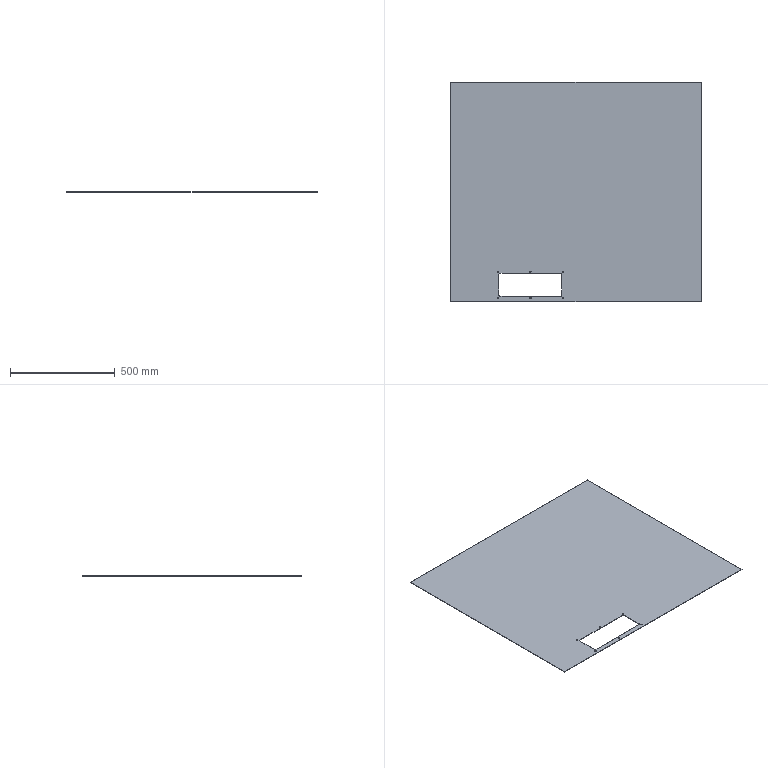Part | SolidWorks | features BaseBody 1 | 1 solid | 26 faces | box 1196 x 1046 x 2 mm | volume 2435677 mm3 | cylinder 16 | plane 10 | commonest cylinder face diameters 6.5 x12 10 x4
STEP:
#1=CARTESIAN_POINT('',(-369.75,-505.5,2.));
#2=VERTEX_POINT('',#1);
#3=CARTESIAN_POINT('',(-369.75,-505.5,0.));
#4=VERTEX_POINT('',#3);
#5=CARTESIAN_POINT('',(-369.75,-505.5,2.));
#6=DIRECTION('',(0.,0.,-1.));
#7=VECTOR('',#6,1000.);
#8=LINE('',#5,#7);
#9=EDGE_CURVE('',#2,#4,#8,.T.);
#10=ORIENTED_EDGE('',*,*,#9,.F.);
#11=CARTESIAN_POINT('',(-376.25,-505.5,2.));
#12=VERTEX_POINT('',#11);
#13=CARTESIAN_POINT('',(-373.,-505.5,2.));
#14=DIRECTION('',(0.,0.,-1.));
#15=DIRECTION('',(1.,0.,0.));
#16=AXIS2_PLACEMENT_3D('',#13,#14,#15);
#17=CIRCLE('',#16,3.25);
#18=EDGE_CURVE('',#12,#2,#17,.T.);
#19=ORIENTED_EDGE('',*,*,#18,.F.);
#20=CARTESIAN_POINT('',(-376.25,-505.5,0.));
#21=VERTEX_POINT('',#20);
#22=CARTESIAN_POINT('',(-376.25,-505.5,2.));
#23=DIRECTION('',(0.,0.,-1.));
#24=VECTOR('',#23,1000.);
#25=LINE('',#22,#24);
#26=EDGE_CURVE('',#12,#21,#25,.T.);
#27=ORIENTED_EDGE('',*,*,#26,.T.);
#28=CARTESIAN_POINT('',(-373.,-505.5,0.));
#29=DIRECTION('',(0.,0.,-1.));
#30=DIRECTION('',(1.,0.,0.));
#31=AXIS2_PLACEMENT_3D('',#28,#29,#30);
#32=CIRCLE('',#31,3.25);
#33=EDGE_CURVE('',#21,#4,#32,.T.);
#34=ORIENTED_EDGE('',*,*,#33,.T.);
#35=EDGE_LOOP('',(#10,#19,#27,#34));
#36=FACE_OUTER_BOUND('',#35,.T.);
#37=CARTESIAN_POINT('',(-373.,-505.5,2.));
#38=DIRECTION('',(0.,0.,-1.));
#39=DIRECTION('',(-1.,0.,0.));
#40=AXIS2_PLACEMENT_3D('',#37,#38,#39);
#41=CYLINDRICAL_SURFACE('',#40,3.25);
#42=ADVANCED_FACE('',(#36),#41,.F.);
#43=CARTESIAN_POINT('',(-214.75,-505.5,2.));
#44=VERTEX_POINT('',#43);
#45=CARTESIAN_POINT('',(-214.75,-505.5,0.));
#46=VERTEX_POINT('',#45);
#47=CARTESIAN_POINT('',(-214.75,-505.5,2.));
#48=DIRECTION('',(0.,0.,-1.));
#49=VECTOR('',#48,1000.);
#50=LINE('',#47,#49);
#51=EDGE_CURVE('',#44,#46,#50,.T.);
#52=ORIENTED_EDGE('',*,*,#51,.F.);
#53=CARTESIAN_POINT('',(-221.25,-505.5,2.));
#54=VERTEX_POINT('',#53);
#55=CARTESIAN_POINT('',(-218.,-505.5,2.));
#56=DIRECTION('',(0.,0.,-1.));
#57=DIRECTION('',(-1.,0.,0.));
#58=AXIS2_PLACEMENT_3D('',#55,#56,#57);
#59=CIRCLE('',#58,3.25);
#60=EDGE_CURVE('',#54,#44,#59,.T.);
#61=ORIENTED_EDGE('',*,*,#60,.F.);
#62=CARTESIAN_POINT('',(-221.25,-505.5,0.));
#63=VERTEX_POINT('',#62);
#64=CARTESIAN_POINT('',(-221.25,-505.5,2.));
#65=DIRECTION('',(0.,0.,-1.));
#66=VECTOR('',#65,1000.);
#67=LINE('',#64,#66);
#68=EDGE_CURVE('',#54,#63,#67,.T.);
#69=ORIENTED_EDGE('',*,*,#68,.T.);
#70=CARTESIAN_POINT('',(-218.,-505.5,0.));
#71=DIRECTION('',(0.,0.,-1.));
#72=DIRECTION('',(-1.,0.,0.));
#73=AXIS2_PLACEMENT_3D('',#70,#71,#72);
#74=CIRCLE('',#73,3.25);
#75=EDGE_CURVE('',#63,#46,#74,.T.);
#76=ORIENTED_EDGE('',*,*,#75,.T.);
#77=EDGE_LOOP('',(#52,#61,#69,#76));
#78=FACE_OUTER_BOUND('',#77,.T.);
#79=CARTESIAN_POINT('',(-218.,-505.5,2.));
#80=DIRECTION('',(0.,0.,-1.));
#81=DIRECTION('',(-1.,0.,0.));
#82=AXIS2_PLACEMENT_3D('',#79,#80,#81);
#83=CYLINDRICAL_SURFACE('',#82,3.25);
#84=ADVANCED_FACE('',(#78),#83,.F.);
#85=CARTESIAN_POINT('',(-214.75,-380.5,2.));
#86=VERTEX_POINT('',#85);
#87=CARTESIAN_POINT('',(-214.75,-380.5,0.));
#88=VERTEX_POINT('',#87);
#89=CARTESIAN_POINT('',(-214.75,-380.5,2.));
#90=DIRECTION('',(0.,0.,-1.));
#91=VECTOR('',#90,1000.);
#92=LINE('',#89,#91);
#93=EDGE_CURVE('',#86,#88,#92,.T.);
#94=ORIENTED_EDGE('',*,*,#93,.F.);
#95=CARTESIAN_POINT('',(-221.25,-380.5,2.));
#96=VERTEX_POINT('',#95);
#97=CARTESIAN_POINT('',(-218.,-380.5,2.));
#98=DIRECTION('',(0.,0.,-1.));
#99=DIRECTION('',(-1.,0.,0.));
#100=AXIS2_PLACEMENT_3D('',#97,#98,#99);
#101=CIRCLE('',#100,3.25);
#102=EDGE_CURVE('',#96,#86,#101,.T.);
#103=ORIENTED_EDGE('',*,*,#102,.F.);
#104=CARTESIAN_POINT('',(-221.25,-380.5,0.));
#105=VERTEX_POINT('',#104);
#106=CARTESIAN_POINT('',(-221.25,-380.5,2.));
#107=DIRECTION('',(0.,0.,-1.));
#108=VECTOR('',#107,1000.);
#109=LINE('',#106,#108);
#110=EDGE_CURVE('',#96,#105,#109,.T.);
#111=ORIENTED_EDGE('',*,*,#110,.T.);
#112=CARTESIAN_POINT('',(-218.,-380.5,0.));
#113=DIRECTION('',(0.,0.,-1.));
#114=DIRECTION('',(-1.,0.,0.));
#115=AXIS2_PLACEMENT_3D('',#112,#113,#114);
#116=CIRCLE('',#115,3.25);
#117=EDGE_CURVE('',#105,#88,#116,.T.);
#118=ORIENTED_EDGE('',*,*,#117,.T.);
#119=EDGE_LOOP('',(#94,#103,#111,#118));
#120=FACE_OUTER_BOUND('',#119,.T.);
#121=CARTESIAN_POINT('',(-218.,-380.5,2.));
#122=DIRECTION('',(0.,0.,-1.));
#123=DIRECTION('',(-1.,0.,0.));
#124=AXIS2_PLACEMENT_3D('',#121,#122,#123);
#125=CYLINDRICAL_SURFACE('',#124,3.25);
#126=ADVANCED_FACE('',(#120),#125,.F.);
#127=CARTESIAN_POINT('',(-59.75,-505.5,2.));
#128=VERTEX_POINT('',#127);
#129=CARTESIAN_POINT('',(-59.75,-505.5,0.));
#130=VERTEX_POINT('',#129);
#131=CARTESIAN_POINT('',(-59.75,-505.5,2.));
#132=DIRECTION('',(0.,0.,-1.));
#133=VECTOR('',#132,1000.);
#134=LINE('',#131,#133);
#135=EDGE_CURVE('',#128,#130,#134,.T.);
#136=ORIENTED_EDGE('',*,*,#135,.F.);
#137=CARTESIAN_POINT('',(-66.25,-505.5,2.));
#138=VERTEX_POINT('',#137);
#139=CARTESIAN_POINT('',(-63.,-505.5,2.));
#140=DIRECTION('',(0.,0.,-1.));
#141=DIRECTION('',(-1.,0.,0.));
#142=AXIS2_PLACEMENT_3D('',#139,#140,#141);
#143=CIRCLE('',#142,3.25);
#144=EDGE_CURVE('',#138,#128,#143,.T.);
#145=ORIENTED_EDGE('',*,*,#144,.F.);
#146=CARTESIAN_POINT('',(-66.25,-505.5,0.));
#147=VERTEX_POINT('',#146);
#148=CARTESIAN_POINT('',(-66.25,-505.5,2.));
#149=DIRECTION('',(0.,0.,-1.));
#150=VECTOR('',#149,1000.);
#151=LINE('',#148,#150);
#152=EDGE_CURVE('',#138,#147,#151,.T.);
#153=ORIENTED_EDGE('',*,*,#152,.T.);
#154=CARTESIAN_POINT('',(-63.,-505.5,0.));
#155=DIRECTION('',(0.,0.,-1.));
#156=DIRECTION('',(-1.,0.,0.));
#157=AXIS2_PLACEMENT_3D('',#154,#155,#156);
#158=CIRCLE('',#157,3.25);
#159=EDGE_CURVE('',#147,#130,#158,.T.);
#160=ORIENTED_EDGE('',*,*,#159,.T.);
#161=EDGE_LOOP('',(#136,#145,#153,#160));
#162=FACE_OUTER_BOUND('',#161,.T.);
#163=CARTESIAN_POINT('',(-63.,-505.5,2.));
#164=DIRECTION('',(0.,0.,-1.));
#165=DIRECTION('',(-1.,0.,0.));
#166=AXIS2_PLACEMENT_3D('',#163,#164,#165);
#167=CYLINDRICAL_SURFACE('',#166,3.25);
#168=ADVANCED_FACE('',(#162),#167,.F.);
#169=CARTESIAN_POINT('',(-369.75,-380.5,2.));
#170=VERTEX_POINT('',#169);
#171=CARTESIAN_POINT('',(-369.75,-380.5,0.));
#172=VERTEX_POINT('',#171);
#173=CARTESIAN_POINT('',(-369.75,-380.5,2.));
#174=DIRECTION('',(0.,0.,-1.));
#175=VECTOR('',#174,1000.);
#176=LINE('',#173,#175);
#177=EDGE_CURVE('',#170,#172,#176,.T.);
#178=ORIENTED_EDGE('',*,*,#177,.F.);
#179=CARTESIAN_POINT('',(-376.25,-380.5,2.));
#180=VERTEX_POINT('',#179);
#181=CARTESIAN_POINT('',(-373.,-380.5,2.));
#182=DIRECTION('',(0.,0.,-1.));
#183=DIRECTION('',(1.,0.,0.));
#184=AXIS2_PLACEMENT_3D('',#181,#182,#183);
#185=CIRCLE('',#184,3.25);
#186=EDGE_CURVE('',#180,#170,#185,.T.);
#187=ORIENTED_EDGE('',*,*,#186,.F.);
#188=CARTESIAN_POINT('',(-376.25,-380.5,0.));
#189=VERTEX_POINT('',#188);
#190=CARTESIAN_POINT('',(-376.25,-380.5,2.));
#191=DIRECTION('',(0.,0.,-1.));
#192=VECTOR('',#191,1000.);
#193=LINE('',#190,#192);
#194=EDGE_CURVE('',#180,#189,#193,.T.);
#195=ORIENTED_EDGE('',*,*,#194,.T.);
#196=CARTESIAN_POINT('',(-373.,-380.5,0.));
#197=DIRECTION('',(0.,0.,-1.));
#198=DIRECTION('',(1.,0.,0.));
#199=AXIS2_PLACEMENT_3D('',#196,#197,#198);
#200=CIRCLE('',#199,3.25);
#201=EDGE_CURVE('',#189,#172,#200,.T.);
#202=ORIENTED_EDGE('',*,*,#201,.T.);
#203=EDGE_LOOP('',(#178,#187,#195,#202));
#204=FACE_OUTER_BOUND('',#203,.T.);
#205=CARTESIAN_POINT('',(-373.,-380.5,2.));
#206=DIRECTION('',(0.,0.,-1.));
#207=DIRECTION('',(-1.,0.,0.));
#208=AXIS2_PLACEMENT_3D('',#205,#206,#207);
#209=CYLINDRICAL_SURFACE('',#208,3.25);
#210=ADVANCED_FACE('',(#204),#209,.F.);
#211=CARTESIAN_POINT('',(-59.75,-380.5,2.));
#212=VERTEX_POINT('',#211);
#213=CARTESIAN_POINT('',(-59.75,-380.5,0.));
#214=VERTEX_POINT('',#213);
#215=CARTESIAN_POINT('',(-59.75,-380.5,2.));
#216=DIRECTION('',(0.,0.,-1.));
#217=VECTOR('',#216,1000.);
#218=LINE('',#215,#217);
#219=EDGE_CURVE('',#212,#214,#218,.T.);
#220=ORIENTED_EDGE('',*,*,#219,.F.);
#221=CARTESIAN_POINT('',(-66.25,-380.5,2.));
#222=VERTEX_POINT('',#221);
#223=CARTESIAN_POINT('',(-63.,-380.5,2.));
#224=DIRECTION('',(0.,0.,-1.));
#225=DIRECTION('',(-1.,0.,0.));
#226=AXIS2_PLACEMENT_3D('',#223,#224,#225);
#227=CIRCLE('',#226,3.25);
#228=EDGE_CURVE('',#222,#212,#227,.T.);
#229=ORIENTED_EDGE('',*,*,#228,.F.);
#230=CARTESIAN_POINT('',(-66.25,-380.5,0.));
#231=VERTEX_POINT('',#230);
#232=CARTESIAN_POINT('',(-66.25,-380.5,2.));
#233=DIRECTION('',(0.,0.,-1.));
#234=VECTOR('',#233,1000.);
#235=LINE('',#232,#234);
#236=EDGE_CURVE('',#222,#231,#235,.T.);
#237=ORIENTED_EDGE('',*,*,#236,.T.);
#238=CARTESIAN_POINT('',(-63.,-380.5,0.));
#239=DIRECTION('',(0.,0.,-1.));
#240=DIRECTION('',(-1.,0.,0.));
#241=AXIS2_PLACEMENT_3D('',#238,#239,#240);
#242=CIRCLE('',#241,3.25);
#243=EDGE_CURVE('',#231,#214,#242,.T.);
#244=ORIENTED_EDGE('',*,*,#243,.T.);
#245=EDGE_LOOP('',(#220,#229,#237,#244));
#246=FACE_OUTER_BOUND('',#245,.T.);
#247=CARTESIAN_POINT('',(-63.,-380.5,2.));
#248=DIRECTION('',(0.,0.,-1.));
#249=DIRECTION('',(-1.,0.,0.));
#250=AXIS2_PLACEMENT_3D('',#247,#248,#249);
#251=CYLINDRICAL_SURFACE('',#250,3.25);
#252=ADVANCED_FACE('',(#246),#251,.F.);
#253=CARTESIAN_POINT('',(-73.,-388.,2.));
#254=VERTEX_POINT('',#253);
#255=CARTESIAN_POINT('',(-68.,-393.,2.));
#256=VERTEX_POINT('',#255);
#257=CARTESIAN_POINT('',(-73.,-393.,2.));
#258=DIRECTION('',(0.,0.,-1.));
#259=DIRECTION('',(-1.,0.,0.));
#260=AXIS2_PLACEMENT_3D('',#257,#258,#259);
#261=CIRCLE('',#260,5.);
#262=EDGE_CURVE('',#254,#256,#261,.T.);
#263=ORIENTED_EDGE('',*,*,#262,.F.);
#264=CARTESIAN_POINT('',(-73.,-388.,0.));
#265=VERTEX_POINT('',#264);
#266=CARTESIAN_POINT('',(-73.,-388.,2.));
#267=DIRECTION('',(0.,0.,1.));
#268=VECTOR('',#267,1000.);
#269=LINE('',#266,#268);
#270=EDGE_CURVE('',#265,#254,#269,.T.);
#271=ORIENTED_EDGE('',*,*,#270,.F.);
#272=CARTESIAN_POINT('',(-68.,-393.,0.));
#273=VERTEX_POINT('',#272);
#274=CARTESIAN_POINT('',(-73.,-393.,0.));
#275=DIRECTION('',(0.,0.,1.));
#276=DIRECTION('',(-1.,0.,0.));
#277=AXIS2_PLACEMENT_3D('',#274,#275,#276);
#278=CIRCLE('',#277,5.);
#279=EDGE_CURVE('',#273,#265,#278,.T.);
#280=ORIENTED_EDGE('',*,*,#279,.F.);
#281=CARTESIAN_POINT('',(-68.,-393.,0.));
#282=DIRECTION('',(0.,0.,-1.));
#283=VECTOR('',#282,1000.);
#284=LINE('',#281,#283);
#285=EDGE_CURVE('',#256,#273,#284,.T.);
#286=ORIENTED_EDGE('',*,*,#285,.F.);
#287=EDGE_LOOP('',(#263,#271,#280,#286));
#288=FACE_OUTER_BOUND('',#287,.T.);
#289=CARTESIAN_POINT('',(-73.,-393.,10.));
#290=DIRECTION('',(0.,0.,1.));
#291=DIRECTION('',(1.,0.,0.));
#292=AXIS2_PLACEMENT_3D('',#289,#290,#291);
#293=CYLINDRICAL_SURFACE('',#292,5.);
#294=ADVANCED_FACE('',(#288),#293,.F.);
#295=CARTESIAN_POINT('',(-68.,-493.,2.));
#296=VERTEX_POINT('',#295);
#297=CARTESIAN_POINT('',(-73.,-498.,2.));
#298=VERTEX_POINT('',#297);
#299=CARTESIAN_POINT('',(-73.,-493.,2.));
#300=DIRECTION('',(0.,0.,-1.));
#301=DIRECTION('',(-1.,0.,0.));
#302=AXIS2_PLACEMENT_3D('',#299,#300,#301);
#303=CIRCLE('',#302,5.);
#304=EDGE_CURVE('',#296,#298,#303,.T.);
#305=ORIENTED_EDGE('',*,*,#304,.F.);
#306=CARTESIAN_POINT('',(-68.,-493.,0.));
#307=VERTEX_POINT('',#306);
#308=CARTESIAN_POINT('',(-68.,-493.,2.));
#309=DIRECTION('',(0.,0.,1.));
#310=VECTOR('',#309,1000.);
#311=LINE('',#308,#310);
#312=EDGE_CURVE('',#307,#296,#311,.T.);
#313=ORIENTED_EDGE('',*,*,#312,.F.);
#314=CARTESIAN_POINT('',(-73.,-498.,0.));
#315=VERTEX_POINT('',#314);
#316=CARTESIAN_POINT('',(-73.,-493.,0.));
#317=DIRECTION('',(0.,0.,1.));
#318=DIRECTION('',(-1.,0.,0.));
#319=AXIS2_PLACEMENT_3D('',#316,#317,#318);
#320=CIRCLE('',#319,5.);
#321=EDGE_CURVE('',#315,#307,#320,.T.);
#322=ORIENTED_EDGE('',*,*,#321,.F.);
#323=CARTESIAN_POINT('',(-73.,-498.,0.));
#324=DIRECTION('',(0.,0.,-1.));
#325=VECTOR('',#324,1000.);
#326=LINE('',#323,#325);
#327=EDGE_CURVE('',#298,#315,#326,.T.);
#328=ORIENTED_EDGE('',*,*,#327,.F.);
#329=EDGE_LOOP('',(#305,#313,#322,#328));
#330=FACE_OUTER_BOUND('',#329,.T.);
#331=CARTESIAN_POINT('',(-73.,-493.,10.));
#332=DIRECTION('',(0.,0.,1.));
#333=DIRECTION('',(1.,0.,0.));
#334=AXIS2_PLACEMENT_3D('',#331,#332,#333);
#335=CYLINDRICAL_SURFACE('',#334,5.);
#336=ADVANCED_FACE('',(#330),#335,.F.);
#337=CARTESIAN_POINT('',(-368.,-393.,2.));
#338=VERTEX_POINT('',#337);
#339=CARTESIAN_POINT('',(-363.,-388.,2.));
#340=VERTEX_POINT('',#339);
#341=CARTESIAN_POINT('',(-363.,-393.,2.));
#342=DIRECTION('',(0.,0.,-1.));
#343=DIRECTION('',(-1.,0.,0.));
#344=AXIS2_PLACEMENT_3D('',#341,#342,#343);
#345=CIRCLE('',#344,5.);
#346=EDGE_CURVE('',#338,#340,#345,.T.);
#347=ORIENTED_EDGE('',*,*,#346,.F.);
#348=CARTESIAN_POINT('',(-368.,-393.,0.));
#349=VERTEX_POINT('',#348);
#350=CARTESIAN_POINT('',(-368.,-393.,2.));
#351=DIRECTION('',(0.,0.,1.));
#352=VECTOR('',#351,1000.);
#353=LINE('',#350,#352);
#354=EDGE_CURVE('',#349,#338,#353,.T.);
#355=ORIENTED_EDGE('',*,*,#354,.F.);
#356=CARTESIAN_POINT('',(-363.,-388.,0.));
#357=VERTEX_POINT('',#356);
#358=CARTESIAN_POINT('',(-363.,-393.,0.));
#359=DIRECTION('',(0.,0.,1.));
#360=DIRECTION('',(-1.,0.,0.));
#361=AXIS2_PLACEMENT_3D('',#358,#359,#360);
#362=CIRCLE('',#361,5.);
#363=EDGE_CURVE('',#357,#349,#362,.T.);
#364=ORIENTED_EDGE('',*,*,#363,.F.);
#365=CARTESIAN_POINT('',(-363.,-388.,0.));
#366=DIRECTION('',(0.,0.,-1.));
#367=VECTOR('',#366,1000.);
#368=LINE('',#365,#367);
#369=EDGE_CURVE('',#340,#357,#368,.T.);
#370=ORIENTED_EDGE('',*,*,#369,.F.);
#371=EDGE_LOOP('',(#347,#355,#364,#370));
#372=FACE_OUTER_BOUND('',#371,.T.);
#373=CARTESIAN_POINT('',(-363.,-393.,10.));
#374=DIRECTION('',(0.,0.,1.));
#375=DIRECTION('',(1.,0.,0.));
#376=AXIS2_PLACEMENT_3D('',#373,#374,#375);
#377=CYLINDRICAL_SURFACE('',#376,5.);
#378=ADVANCED_FACE('',(#372),#377,.F.);
#379=CARTESIAN_POINT('',(-363.,-498.,2.));
#380=VERTEX_POINT('',#379);
#381=CARTESIAN_POINT('',(-368.,-493.,2.));
#382=VERTEX_POINT('',#381);
#383=CARTESIAN_POINT('',(-363.,-493.,2.));
#384=DIRECTION('',(0.,0.,-1.));
#385=DIRECTION('',(-1.,0.,0.));
#386=AXIS2_PLACEMENT_3D('',#383,#384,#385);
#387=CIRCLE('',#386,5.);
#388=EDGE_CURVE('',#380,#382,#387,.T.);
#389=ORIENTED_EDGE('',*,*,#388,.F.);
#390=CARTESIAN_POINT('',(-363.,-498.,0.));
#391=VERTEX_POINT('',#390);
#392=CARTESIAN_POINT('',(-363.,-498.,2.));
#393=DIRECTION('',(0.,0.,1.));
#394=VECTOR('',#393,1000.);
#395=LINE('',#392,#394);
#396=EDGE_CURVE('',#391,#380,#395,.T.);
#397=ORIENTED_EDGE('',*,*,#396,.F.);
#398=CARTESIAN_POINT('',(-368.,-493.,0.));
#399=VERTEX_POINT('',#398);
#400=CARTESIAN_POINT('',(-363.,-493.,0.));
#401=DIRECTION('',(0.,0.,1.));
#402=DIRECTION('',(-1.,0.,0.));
#403=AXIS2_PLACEMENT_3D('',#400,#401,#402);
#404=CIRCLE('',#403,5.);
#405=EDGE_CURVE('',#399,#391,#404,.T.);
#406=ORIENTED_EDGE('',*,*,#405,.F.);
#407=CARTESIAN_POINT('',(-368.,-493.,0.));
#408=DIRECTION('',(0.,0.,-1.));
#409=VECTOR('',#408,1000.);
#410=LINE('',#407,#409);
#411=EDGE_CURVE('',#382,#399,#410,.T.);
#412=ORIENTED_EDGE('',*,*,#411,.F.);
#413=EDGE_LOOP('',(#389,#397,#406,#412));
#414=FACE_OUTER_BOUND('',#413,.T.);
#415=CARTESIAN_POINT('',(-363.,-493.,10.));
#416=DIRECTION('',(0.,0.,1.));
#417=DIRECTION('',(1.,0.,0.));
#418=AXIS2_PLACEMENT_3D('',#415,#416,#417);
#419=CYLINDRICAL_SURFACE('',#418,5.);
#420=ADVANCED_FACE('',(#414),#419,.F.);
#421=CARTESIAN_POINT('',(-368.,-498.,0.));
#422=DIRECTION('',(-1.,0.,0.));
#423=VECTOR('',#422,1000.);
#424=LINE('',#421,#423);
#425=EDGE_CURVE('',#315,#391,#424,.T.);
#426=ORIENTED_EDGE('',*,*,#425,.T.);
#427=ORIENTED_EDGE('',*,*,#396,.T.);
#428=CARTESIAN_POINT('',(0.,-498.,2.));
#429=DIRECTION('',(-1.,0.,0.));
#430=VECTOR('',#429,1000.);
#431=LINE('',#428,#430);
#432=EDGE_CURVE('',#298,#380,#431,.T.);
#433=ORIENTED_EDGE('',*,*,#432,.F.);
#434=ORIENTED_EDGE('',*,*,#327,.T.);
#435=EDGE_LOOP('',(#426,#427,#433,#434));
#436=FACE_OUTER_BOUND('',#435,.T.);
#437=CARTESIAN_POINT('',(-368.,-498.,10.));
#438=DIRECTION('',(0.,-1.,0.));
#439=DIRECTION('',(-1.,0.,0.));
#440=AXIS2_PLACEMENT_3D('',#437,#438,#439);
#441=PLANE('',#440);
#442=ADVANCED_FACE('',(#436),#441,.F.);
#443=CARTESIAN_POINT('',(-368.,0.,2.));
#444=DIRECTION('',(0.,1.,0.));
#445=VECTOR('',#444,1000.);
#446=LINE('',#443,#445);
#447=EDGE_CURVE('',#382,#338,#446,.T.);
#448=ORIENTED_EDGE('',*,*,#447,.F.);
#449=ORIENTED_EDGE('',*,*,#411,.T.);
#450=CARTESIAN_POINT('',(-368.,-388.,0.));
#451=DIRECTION('',(0.,1.,0.));
#452=VECTOR('',#451,1000.);
#453=LINE('',#450,#452);
#454=EDGE_CURVE('',#399,#349,#453,.T.);
#455=ORIENTED_EDGE('',*,*,#454,.T.);
#456=ORIENTED_EDGE('',*,*,#354,.T.);
#457=EDGE_LOOP('',(#448,#449,#455,#456));
#458=FACE_OUTER_BOUND('',#457,.T.);
#459=CARTESIAN_POINT('',(-368.,-388.,10.));
#460=DIRECTION('',(-1.,0.,0.));
#461=DIRECTION('',(0.,0.,1.));
#462=AXIS2_PLACEMENT_3D('',#459,#460,#461);
#463=PLANE('',#462);
#464=ADVANCED_FACE('',(#458),#463,.F.);
#465=CARTESIAN_POINT('',(0.,-388.,2.));
#466=DIRECTION('',(1.,0.,0.));
#467=VECTOR('',#466,1000.);
#468=LINE('',#465,#467);
#469=EDGE_CURVE('',#340,#254,#468,.T.);
#470=ORIENTED_EDGE('',*,*,#469,.F.);
#471=ORIENTED_EDGE('',*,*,#369,.T.);
#472=CARTESIAN_POINT('',(-368.,-388.,0.));
#473=DIRECTION('',(1.,0.,0.));
#474=VECTOR('',#473,1000.);
#475=LINE('',#472,#474);
#476=EDGE_CURVE('',#357,#265,#475,.T.);
#477=ORIENTED_EDGE('',*,*,#476,.T.);
#478=ORIENTED_EDGE('',*,*,#270,.T.);
#479=EDGE_LOOP('',(#470,#471,#477,#478));
#480=FACE_OUTER_BOUND('',#479,.T.);
#481=CARTESIAN_POINT('',(-368.,-388.,10.));
#482=DIRECTION('',(0.,1.,0.));
#483=DIRECTION('',(1.,0.,0.));
#484=AXIS2_PLACEMENT_3D('',#481,#482,#483);
#485=PLANE('',#484);
#486=ADVANCED_FACE('',(#480),#485,.F.);
#487=CARTESIAN_POINT('',(-68.,-388.,0.));
#488=DIRECTION('',(0.,-1.,0.));
#489=VECTOR('',#488,1000.);
#490=LINE('',#487,#489);
#491=EDGE_CURVE('',#273,#307,#490,.T.);
#492=ORIENTED_EDGE('',*,*,#491,.T.);
#493=ORIENTED_EDGE('',*,*,#312,.T.);
#494=CARTESIAN_POINT('',(-68.,0.,2.));
#495=DIRECTION('',(0.,-1.,0.));
#496=VECTOR('',#495,1000.);
#497=LINE('',#494,#496);
#498=EDGE_CURVE('',#256,#296,#497,.T.);
#499=ORIENTED_EDGE('',*,*,#498,.F.);
#500=ORIENTED_EDGE('',*,*,#285,.T.);
#501=EDGE_LOOP('',(#492,#493,#499,#500));
#502=FACE_OUTER_BOUND('',#501,.T.);
#503=CARTESIAN_POINT('',(-68.,-388.,10.));
#504=DIRECTION('',(1.,0.,0.));
#505=DIRECTION('',(0.,1.,0.));
#506=AXIS2_PLACEMENT_3D('',#503,#504,#505);
#507=PLANE('',#506);
#508=ADVANCED_FACE('',(#502),#507,.F.);
#509=ORIENTED_EDGE('',*,*,#491,.F.);
#510=ORIENTED_EDGE('',*,*,#279,.T.);
#511=ORIENTED_EDGE('',*,*,#476,.F.);
#512=ORIENTED_EDGE('',*,*,#363,.T.);
#513=ORIENTED_EDGE('',*,*,#454,.F.);
#514=ORIENTED_EDGE('',*,*,#405,.T.);
#515=ORIENTED_EDGE('',*,*,#425,.F.);
#516=ORIENTED_EDGE('',*,*,#321,.T.);
#517=EDGE_LOOP('',(#509,#510,#511,#512,#513,#514,#515,#516));
#518=FACE_BOUND('',#517,.T.);
#519=ORIENTED_EDGE('',*,*,#243,.F.);
#520=CARTESIAN_POINT('',(-63.,-380.5,0.));
#521=DIRECTION('',(0.,0.,-1.));
#522=DIRECTION('',(-1.,0.,0.));
#523=AXIS2_PLACEMENT_3D('',#520,#521,#522);
#524=CIRCLE('',#523,3.25);
#525=EDGE_CURVE('',#214,#231,#524,.T.);
#526=ORIENTED_EDGE('',*,*,#525,.F.);
#527=EDGE_LOOP('',(#519,#526));
#528=FACE_BOUND('',#527,.T.);
#529=ORIENTED_EDGE('',*,*,#201,.F.);
#530=CARTESIAN_POINT('',(-373.,-380.5,0.));
#531=DIRECTION('',(0.,0.,-1.));
#532=DIRECTION('',(1.,0.,0.));
#533=AXIS2_PLACEMENT_3D('',#530,#531,#532);
#534=CIRCLE('',#533,3.25);
#535=EDGE_CURVE('',#172,#189,#534,.T.);
#536=ORIENTED_EDGE('',*,*,#535,.F.);
#537=EDGE_LOOP('',(#529,#536));
#538=FACE_BOUND('',#537,.T.);
#539=ORIENTED_EDGE('',*,*,#159,.F.);
#540=CARTESIAN_POINT('',(-63.,-505.5,0.));
#541=DIRECTION('',(0.,0.,-1.));
#542=DIRECTION('',(-1.,0.,0.));
#543=AXIS2_PLACEMENT_3D('',#540,#541,#542);
#544=CIRCLE('',#543,3.25);
#545=EDGE_CURVE('',#130,#147,#544,.T.);
#546=ORIENTED_EDGE('',*,*,#545,.F.);
#547=EDGE_LOOP('',(#539,#546));
#548=FACE_BOUND('',#547,.T.);
#549=ORIENTED_EDGE('',*,*,#117,.F.);
#550=CARTESIAN_POINT('',(-218.,-380.5,0.));
#551=DIRECTION('',(0.,0.,-1.));
#552=DIRECTION('',(-1.,0.,0.));
#553=AXIS2_PLACEMENT_3D('',#550,#551,#552);
#554=CIRCLE('',#553,3.25);
#555=EDGE_CURVE('',#88,#105,#554,.T.);
#556=ORIENTED_EDGE('',*,*,#555,.F.);
#557=EDGE_LOOP('',(#549,#556));
#558=FACE_BOUND('',#557,.T.);
#559=ORIENTED_EDGE('',*,*,#75,.F.);
#560=CARTESIAN_POINT('',(-218.,-505.5,0.));
#561=DIRECTION('',(0.,0.,-1.));
#562=DIRECTION('',(-1.,0.,0.));
#563=AXIS2_PLACEMENT_3D('',#560,#561,#562);
#564=CIRCLE('',#563,3.25);
#565=EDGE_CURVE('',#46,#63,#564,.T.);
#566=ORIENTED_EDGE('',*,*,#565,.F.);
#567=EDGE_LOOP('',(#559,#566));
#568=FACE_BOUND('',#567,.T.);
#569=ORIENTED_EDGE('',*,*,#33,.F.);
#570=CARTESIAN_POINT('',(-373.,-505.5,0.));
#571=DIRECTION('',(0.,0.,-1.));
#572=DIRECTION('',(1.,0.,0.));
#573=AXIS2_PLACEMENT_3D('',#570,#571,#572);
#574=CIRCLE('',#573,3.25);
#575=EDGE_CURVE('',#4,#21,#574,.T.);
#576=ORIENTED_EDGE('',*,*,#575,.F.);
#577=EDGE_LOOP('',(#569,#576));
#578=FACE_BOUND('',#577,.T.);
#579=CARTESIAN_POINT('',(-598.,523.,0.));
#580=VERTEX_POINT('',#579);
#581=CARTESIAN_POINT('',(-598.,-523.,0.));
#582=VERTEX_POINT('',#581);
#583=CARTESIAN_POINT('',(-598.,523.,0.));
#584=DIRECTION('',(0.,-1.,0.));
#585=VECTOR('',#584,1000.);
#586=LINE('',#583,#585);
#587=EDGE_CURVE('',#580,#582,#586,.T.);
#588=ORIENTED_EDGE('',*,*,#587,.F.);
#589=CARTESIAN_POINT('',(598.,523.,0.));
#590=VERTEX_POINT('',#589);
#591=CARTESIAN_POINT('',(598.,523.,0.));
#592=DIRECTION('',(-1.,0.,0.));
#593=VECTOR('',#592,1000.);
#594=LINE('',#591,#593);
#595=EDGE_CURVE('',#590,#580,#594,.T.);
#596=ORIENTED_EDGE('',*,*,#595,.F.);
#597=CARTESIAN_POINT('',(598.,-523.,0.));
#598=VERTEX_POINT('',#597);
#599=CARTESIAN_POINT('',(598.,523.,0.));
#600=DIRECTION('',(0.,1.,0.));
#601=VECTOR('',#600,1000.);
#602=LINE('',#599,#601);
#603=EDGE_CURVE('',#598,#590,#602,.T.);
#604=ORIENTED_EDGE('',*,*,#603,.F.);
#605=CARTESIAN_POINT('',(598.,-523.,0.));
#606=DIRECTION('',(1.,0.,0.));
#607=VECTOR('',#606,1000.);
#608=LINE('',#605,#607);
#609=EDGE_CURVE('',#582,#598,#608,.T.);
#610=ORIENTED_EDGE('',*,*,#609,.F.);
#611=EDGE_LOOP('',(#588,#596,#604,#610));
#612=FACE_OUTER_BOUND('',#611,.T.);
#613=CARTESIAN_POINT('',(0.,0.,0.));
#614=DIRECTION('',(0.,0.,-1.));
#615=DIRECTION('',(0.,-1.,0.));
#616=AXIS2_PLACEMENT_3D('',#613,#614,#615);
#617=PLANE('',#616);
#618=ADVANCED_FACE('',(#518,#528,#538,#548,#558,#568,#578,#612),#617,.T.);
#619=ORIENTED_EDGE('',*,*,#447,.T.);
#620=ORIENTED_EDGE('',*,*,#346,.T.);
#621=ORIENTED_EDGE('',*,*,#469,.T.);
#622=ORIENTED_EDGE('',*,*,#262,.T.);
#623=ORIENTED_EDGE('',*,*,#498,.T.);
#624=ORIENTED_EDGE('',*,*,#304,.T.);
#625=ORIENTED_EDGE('',*,*,#432,.T.);
#626=ORIENTED_EDGE('',*,*,#388,.T.);
#627=EDGE_LOOP('',(#619,#620,#621,#622,#623,#624,#625,#626));
#628=FACE_BOUND('',#627,.T.);
#629=ORIENTED_EDGE('',*,*,#228,.T.);
#630=CARTESIAN_POINT('',(-63.,-380.5,2.));
#631=DIRECTION('',(0.,0.,-1.));
#632=DIRECTION('',(-1.,0.,0.));
#633=AXIS2_PLACEMENT_3D('',#630,#631,#632);
#634=CIRCLE('',#633,3.25);
#635=EDGE_CURVE('',#212,#222,#634,.T.);
#636=ORIENTED_EDGE('',*,*,#635,.T.);
#637=EDGE_LOOP('',(#629,#636));
#638=FACE_BOUND('',#637,.T.);
#639=ORIENTED_EDGE('',*,*,#186,.T.);
#640=CARTESIAN_POINT('',(-373.,-380.5,2.));
#641=DIRECTION('',(0.,0.,-1.));
#642=DIRECTION('',(1.,0.,0.));
#643=AXIS2_PLACEMENT_3D('',#640,#641,#642);
#644=CIRCLE('',#643,3.25);
#645=EDGE_CURVE('',#170,#180,#644,.T.);
#646=ORIENTED_EDGE('',*,*,#645,.T.);
#647=EDGE_LOOP('',(#639,#646));
#648=FACE_BOUND('',#647,.T.);
#649=ORIENTED_EDGE('',*,*,#144,.T.);
#650=CARTESIAN_POINT('',(-63.,-505.5,2.));
#651=DIRECTION('',(0.,0.,-1.));
#652=DIRECTION('',(-1.,0.,0.));
#653=AXIS2_PLACEMENT_3D('',#650,#651,#652);
#654=CIRCLE('',#653,3.25);
#655=EDGE_CURVE('',#128,#138,#654,.T.);
#656=ORIENTED_EDGE('',*,*,#655,.T.);
#657=EDGE_LOOP('',(#649,#656));
#658=FACE_BOUND('',#657,.T.);
#659=ORIENTED_EDGE('',*,*,#102,.T.);
#660=CARTESIAN_POINT('',(-218.,-380.5,2.));
#661=DIRECTION('',(0.,0.,-1.));
#662=DIRECTION('',(-1.,0.,0.));
#663=AXIS2_PLACEMENT_3D('',#660,#661,#662);
#664=CIRCLE('',#663,3.25);
#665=EDGE_CURVE('',#86,#96,#664,.T.);
#666=ORIENTED_EDGE('',*,*,#665,.T.);
#667=EDGE_LOOP('',(#659,#666));
#668=FACE_BOUND('',#667,.T.);
#669=ORIENTED_EDGE('',*,*,#60,.T.);
#670=CARTESIAN_POINT('',(-218.,-505.5,2.));
#671=DIRECTION('',(0.,0.,-1.));
#672=DIRECTION('',(-1.,0.,0.));
#673=AXIS2_PLACEMENT_3D('',#670,#671,#672);
#674=CIRCLE('',#673,3.25);
#675=EDGE_CURVE('',#44,#54,#674,.T.);
#676=ORIENTED_EDGE('',*,*,#675,.T.);
#677=EDGE_LOOP('',(#669,#676));
#678=FACE_BOUND('',#677,.T.);
#679=ORIENTED_EDGE('',*,*,#18,.T.);
#680=CARTESIAN_POINT('',(-373.,-505.5,2.));
#681=DIRECTION('',(0.,0.,-1.));
#682=DIRECTION('',(1.,0.,0.));
#683=AXIS2_PLACEMENT_3D('',#680,#681,#682);
#684=CIRCLE('',#683,3.25);
#685=EDGE_CURVE('',#2,#12,#684,.T.);
#686=ORIENTED_EDGE('',*,*,#685,.T.);
#687=EDGE_LOOP('',(#679,#686));
#688=FACE_BOUND('',#687,.T.);
#689=CARTESIAN_POINT('',(-598.,523.,2.));
#690=VERTEX_POINT('',#689);
#691=CARTESIAN_POINT('',(-598.,-523.,2.));
#692=VERTEX_POINT('',#691);
#693=CARTESIAN_POINT('',(-598.,523.,2.));
#694=DIRECTION('',(0.,-1.,0.));
#695=VECTOR('',#694,1000.);
#696=LINE('',#693,#695);
#697=EDGE_CURVE('',#690,#692,#696,.T.);
#698=ORIENTED_EDGE('',*,*,#697,.T.);
#699=CARTESIAN_POINT('',(598.,-523.,2.));
#700=VERTEX_POINT('',#699);
#701=CARTESIAN_POINT('',(598.,-523.,2.));
#702=DIRECTION('',(1.,0.,0.));
#703=VECTOR('',#702,1000.);
#704=LINE('',#701,#703);
#705=EDGE_CURVE('',#692,#700,#704,.T.);
#706=ORIENTED_EDGE('',*,*,#705,.T.);
#707=CARTESIAN_POINT('',(598.,523.,2.));
#708=VERTEX_POINT('',#707);
#709=CARTESIAN_POINT('',(598.,523.,2.));
#710=DIRECTION('',(0.,1.,0.));
#711=VECTOR('',#710,1000.);
#712=LINE('',#709,#711);
#713=EDGE_CURVE('',#700,#708,#712,.T.);
#714=ORIENTED_EDGE('',*,*,#713,.T.);
#715=CARTESIAN_POINT('',(598.,523.,2.));
#716=DIRECTION('',(-1.,0.,0.));
#717=VECTOR('',#716,1000.);
#718=LINE('',#715,#717);
#719=EDGE_CURVE('',#708,#690,#718,.T.);
#720=ORIENTED_EDGE('',*,*,#719,.T.);
#721=EDGE_LOOP('',(#698,#706,#714,#720));
#722=FACE_OUTER_BOUND('',#721,.T.);
#723=CARTESIAN_POINT('',(0.,0.,2.));
#724=DIRECTION('',(0.,0.,-1.));
#725=DIRECTION('',(0.,-1.,0.));
#726=AXIS2_PLACEMENT_3D('',#723,#724,#725);
#727=PLANE('',#726);
#728=ADVANCED_FACE('',(#628,#638,#648,#658,#668,#678,#688,#722),#727,.F.);
#729=ORIENTED_EDGE('',*,*,#595,.T.);
#730=CARTESIAN_POINT('',(-598.,523.,2.));
#731=DIRECTION('',(0.,0.,-1.));
#732=VECTOR('',#731,1000.);
#733=LINE('',#730,#732);
#734=EDGE_CURVE('',#690,#580,#733,.T.);
#735=ORIENTED_EDGE('',*,*,#734,.F.);
#736=ORIENTED_EDGE('',*,*,#719,.F.);
#737=CARTESIAN_POINT('',(598.,523.,2.));
#738=DIRECTION('',(0.,0.,-1.));
#739=VECTOR('',#738,1000.);
#740=LINE('',#737,#739);
#741=EDGE_CURVE('',#708,#590,#740,.T.);
#742=ORIENTED_EDGE('',*,*,#741,.T.);
#743=EDGE_LOOP('',(#729,#735,#736,#742));
#744=FACE_OUTER_BOUND('',#743,.T.);
#745=CARTESIAN_POINT('',(598.,523.,2.));
#746=DIRECTION('',(0.,-1.,0.));
#747=DIRECTION('',(0.,0.,-1.));
#748=AXIS2_PLACEMENT_3D('',#745,#746,#747);
#749=PLANE('',#748);
#750=ADVANCED_FACE('',(#744),#749,.F.);
#751=ORIENTED_EDGE('',*,*,#603,.T.);
#752=ORIENTED_EDGE('',*,*,#741,.F.);
#753=ORIENTED_EDGE('',*,*,#713,.F.);
#754=CARTESIAN_POINT('',(598.,-523.,2.));
#755=DIRECTION('',(0.,0.,-1.));
#756=VECTOR('',#755,1000.);
#757=LINE('',#754,#756);
#758=EDGE_CURVE('',#700,#598,#757,.T.);
#759=ORIENTED_EDGE('',*,*,#758,.T.);
#760=EDGE_LOOP('',(#751,#752,#753,#759));
#761=FACE_OUTER_BOUND('',#760,.T.);
#762=CARTESIAN_POINT('',(598.,523.,2.));
#763=DIRECTION('',(-1.,0.,0.));
#764=DIRECTION('',(0.,1.,0.));
#765=AXIS2_PLACEMENT_3D('',#762,#763,#764);
#766=PLANE('',#765);
#767=ADVANCED_FACE('',(#761),#766,.F.);
#768=ORIENTED_EDGE('',*,*,#609,.T.);
#769=ORIENTED_EDGE('',*,*,#758,.F.);
#770=ORIENTED_EDGE('',*,*,#705,.F.);
#771=CARTESIAN_POINT('',(-598.,-523.,2.));
#772=DIRECTION('',(0.,0.,-1.));
#773=VECTOR('',#772,1000.);
#774=LINE('',#771,#773);
#775=EDGE_CURVE('',#692,#582,#774,.T.);
#776=ORIENTED_EDGE('',*,*,#775,.T.);
#777=EDGE_LOOP('',(#768,#769,#770,#776));
#778=FACE_OUTER_BOUND('',#777,.T.);
#779=CARTESIAN_POINT('',(598.,-523.,2.));
#780=DIRECTION('',(0.,1.,0.));
#781=DIRECTION('',(1.,0.,0.));
#782=AXIS2_PLACEMENT_3D('',#779,#780,#781);
#783=PLANE('',#782);
#784=ADVANCED_FACE('',(#778),#783,.F.);
#785=ORIENTED_EDGE('',*,*,#587,.T.);
#786=ORIENTED_EDGE('',*,*,#775,.F.);
#787=ORIENTED_EDGE('',*,*,#697,.F.);
#788=ORIENTED_EDGE('',*,*,#734,.T.);
#789=EDGE_LOOP('',(#785,#786,#787,#788));
#790=FACE_OUTER_BOUND('',#789,.T.);
#791=CARTESIAN_POINT('',(-598.,523.,2.));
#792=DIRECTION('',(1.,0.,0.));
#793=DIRECTION('',(0.,1.,0.));
#794=AXIS2_PLACEMENT_3D('',#791,#792,#793);
#795=PLANE('',#794);
#796=ADVANCED_FACE('',(#790),#795,.F.);
#797=ORIENTED_EDGE('',*,*,#635,.F.);
#798=ORIENTED_EDGE('',*,*,#219,.T.);
#799=ORIENTED_EDGE('',*,*,#525,.T.);
#800=ORIENTED_EDGE('',*,*,#236,.F.);
#801=EDGE_LOOP('',(#797,#798,#799,#800));
#802=FACE_OUTER_BOUND('',#801,.T.);
#803=CARTESIAN_POINT('',(-63.,-380.5,2.));
#804=DIRECTION('',(0.,0.,-1.));
#805=DIRECTION('',(-1.,0.,0.));
#806=AXIS2_PLACEMENT_3D('',#803,#804,#805);
#807=CYLINDRICAL_SURFACE('',#806,3.25);
#808=ADVANCED_FACE('',(#802),#807,.F.);
#809=ORIENTED_EDGE('',*,*,#645,.F.);
#810=ORIENTED_EDGE('',*,*,#177,.T.);
#811=ORIENTED_EDGE('',*,*,#535,.T.);
#812=ORIENTED_EDGE('',*,*,#194,.F.);
#813=EDGE_LOOP('',(#809,#810,#811,#812));
#814=FACE_OUTER_BOUND('',#813,.T.);
#815=CARTESIAN_POINT('',(-373.,-380.5,2.));
#816=DIRECTION('',(0.,0.,-1.));
#817=DIRECTION('',(-1.,0.,0.));
#818=AXIS2_PLACEMENT_3D('',#815,#816,#817);
#819=CYLINDRICAL_SURFACE('',#818,3.25);
#820=ADVANCED_FACE('',(#814),#819,.F.);
#821=ORIENTED_EDGE('',*,*,#655,.F.);
#822=ORIENTED_EDGE('',*,*,#135,.T.);
#823=ORIENTED_EDGE('',*,*,#545,.T.);
#824=ORIENTED_EDGE('',*,*,#152,.F.);
#825=EDGE_LOOP('',(#821,#822,#823,#824));
#826=FACE_OUTER_BOUND('',#825,.T.);
#827=CARTESIAN_POINT('',(-63.,-505.5,2.));
#828=DIRECTION('',(0.,0.,-1.));
#829=DIRECTION('',(-1.,0.,0.));
#830=AXIS2_PLACEMENT_3D('',#827,#828,#829);
#831=CYLINDRICAL_SURFACE('',#830,3.25);
#832=ADVANCED_FACE('',(#826),#831,.F.);
#833=ORIENTED_EDGE('',*,*,#665,.F.);
#834=ORIENTED_EDGE('',*,*,#93,.T.);
#835=ORIENTED_EDGE('',*,*,#555,.T.);
#836=ORIENTED_EDGE('',*,*,#110,.F.);
#837=EDGE_LOOP('',(#833,#834,#835,#836));
#838=FACE_OUTER_BOUND('',#837,.T.);
#839=CARTESIAN_POINT('',(-218.,-380.5,2.));
#840=DIRECTION('',(0.,0.,-1.));
#841=DIRECTION('',(-1.,0.,0.));
#842=AXIS2_PLACEMENT_3D('',#839,#840,#841);
#843=CYLINDRICAL_SURFACE('',#842,3.25);
#844=ADVANCED_FACE('',(#838),#843,.F.);
#845=ORIENTED_EDGE('',*,*,#675,.F.);
#846=ORIENTED_EDGE('',*,*,#51,.T.);
#847=ORIENTED_EDGE('',*,*,#565,.T.);
#848=ORIENTED_EDGE('',*,*,#68,.F.);
#849=EDGE_LOOP('',(#845,#846,#847,#848));
#850=FACE_OUTER_BOUND('',#849,.T.);
#851=CARTESIAN_POINT('',(-218.,-505.5,2.));
#852=DIRECTION('',(0.,0.,-1.));
#853=DIRECTION('',(-1.,0.,0.));
#854=AXIS2_PLACEMENT_3D('',#851,#852,#853);
#855=CYLINDRICAL_SURFACE('',#854,3.25);
#856=ADVANCED_FACE('',(#850),#855,.F.);
#857=ORIENTED_EDGE('',*,*,#685,.F.);
#858=ORIENTED_EDGE('',*,*,#9,.T.);
#859=ORIENTED_EDGE('',*,*,#575,.T.);
#860=ORIENTED_EDGE('',*,*,#26,.F.);
#861=EDGE_LOOP('',(#857,#858,#859,#860));
#862=FACE_OUTER_BOUND('',#861,.T.);
#863=CARTESIAN_POINT('',(-373.,-505.5,2.));
#864=DIRECTION('',(0.,0.,-1.));
#865=DIRECTION('',(-1.,0.,0.));
#866=AXIS2_PLACEMENT_3D('',#863,#864,#865);
#867=CYLINDRICAL_SURFACE('',#866,3.25);
#868=ADVANCED_FACE('',(#862),#867,.F.);
#869=CLOSED_SHELL('',(#42,#84,#126,#168,#210,#252,#294,#336,#378,#420,#442,#464,#486,#508,#618,#728,#750,#767,#784,#796,#808,#820,#832,#844,#856,#868));
#870=MANIFOLD_SOLID_BREP('',#869);
#871=CARTESIAN_POINT('',(0.,0.,0.));
#872=DIRECTION('',(0.,0.,1.));
#873=DIRECTION('',(1.,0.,0.));
#874=AXIS2_PLACEMENT_3D('',#871,#872,#873);
#875=(LENGTH_UNIT()NAMED_UNIT(*)SI_UNIT(.MILLI.,.METRE.));
#876=UNCERTAINTY_MEASURE_WITH_UNIT(LENGTH_MEASURE(0.00001),#875,'','');
#877=(NAMED_UNIT(*)PLANE_ANGLE_UNIT()SI_UNIT($,.RADIAN.));
#878=(NAMED_UNIT(*)SI_UNIT($,.STERADIAN.)SOLID_ANGLE_UNIT());
#879=(GEOMETRIC_REPRESENTATION_CONTEXT(3)GLOBAL_UNCERTAINTY_ASSIGNED_CONTEXT((#876))GLOBAL_UNIT_ASSIGNED_CONTEXT((#875,#877,#878))REPRESENTATION_CONTEXT('',''));
#880=ADVANCED_BREP_SHAPE_REPRESENTATION('',(#870,#874),#879);